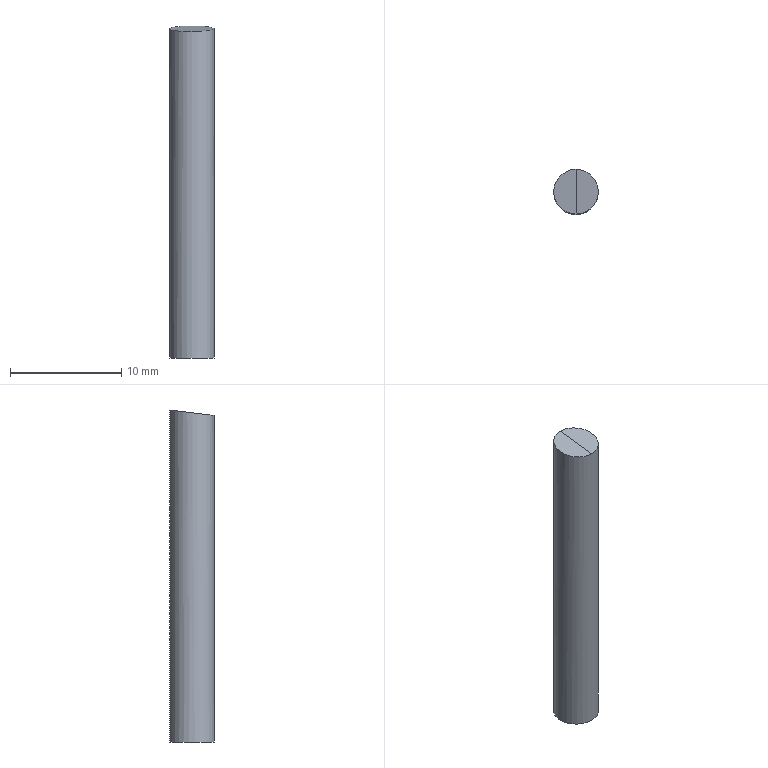Part | NX | features solid 2 | 1 solid | 4 faces | box 4 x 4 x 29.794 mm | volume 371.265 mm3 | plane 3 | cylinder 1 | commonest cylinder face diameters 4 x1
STEP:
#1=CARTESIAN_POINT('',(-0.00002254,-159.993,-1.));
#2=VERTEX_POINT('',#1);
#3=CARTESIAN_POINT('',(-0.00002254,-157.993,-1.));
#4=DIRECTION('',(0.,0.,1.));
#5=DIRECTION('',(0.,-1.,0.));
#6=AXIS2_PLACEMENT_3D('',#3,#4,#5);
#7=CIRCLE('',#6,2.);
#8=EDGE_CURVE('',#2,#2,#7,.T.);
#9=ORIENTED_EDGE('',*,*,#8,.F.);
#10=EDGE_LOOP('',(#9));
#11=FACE_BOUND('',#10,.T.);
#12=CARTESIAN_POINT('',(-0.00002254,-157.993,-1.));
#13=DIRECTION('',(0.,0.,-1.));
#14=DIRECTION('',(0.,1.,0.));
#15=AXIS2_PLACEMENT_3D('',#12,#13,#14);
#16=PLANE('',#15);
#17=ADVANCED_FACE('',(#11),#16,.T.);
#18=ORIENTED_EDGE('',*,*,#8,.T.);
#19=EDGE_LOOP('',(#18));
#20=FACE_BOUND('',#19,.T.);
#21=CARTESIAN_POINT('',(0.,-155.993,28.794));
#22=VERTEX_POINT('',#21);
#23=CARTESIAN_POINT('',(-0.00001127,-159.993,28.295));
#24=VERTEX_POINT('',#23);
#25=CARTESIAN_POINT('',(-0.00002254,-157.993,28.544));
#26=DIRECTION('',(0.,-0.1238,0.9923));
#27=DIRECTION('',(0.,-0.9923,-0.1238));
#28=AXIS2_PLACEMENT_3D('',#25,#26,#27);
#29=ELLIPSE('',#28,2.016,2.);
#30=EDGE_CURVE('',#22,#24,#29,.F.);
#31=ORIENTED_EDGE('',*,*,#30,.T.);
#32=CARTESIAN_POINT('',(-0.00002254,-157.993,28.544));
#33=DIRECTION('',(0.,-0.1238,0.9923));
#34=DIRECTION('',(0.,-0.9923,-0.1238));
#35=AXIS2_PLACEMENT_3D('',#32,#33,#34);
#36=ELLIPSE('',#35,2.016,2.);
#37=EDGE_CURVE('',#24,#22,#36,.F.);
#38=ORIENTED_EDGE('',*,*,#37,.T.);
#39=EDGE_LOOP('',(#31,#38));
#40=FACE_BOUND('',#39,.T.);
#41=CARTESIAN_POINT('',(-0.00002254,-157.993,29.));
#42=DIRECTION('',(0.,0.,-1.));
#43=DIRECTION('',(0.,1.,0.));
#44=AXIS2_PLACEMENT_3D('',#41,#42,#43);
#45=CYLINDRICAL_SURFACE('',#44,2.);
#46=ADVANCED_FACE('',(#20,#40),#45,.T.);
#47=ORIENTED_EDGE('',*,*,#30,.F.);
#48=CARTESIAN_POINT('',(0.,-155.993,28.794));
#49=CARTESIAN_POINT('',(0.,-157.326,28.628));
#50=CARTESIAN_POINT('',(0.,-158.659,28.461));
#51=CARTESIAN_POINT('',(0.,-159.993,28.295));
#52=B_SPLINE_CURVE_WITH_KNOTS('',3,(#48,#49,#50,#51),.UNSPECIFIED.,.F.,.F.,(4,4),(0.4639,0.611),.UNSPECIFIED.);
#53=EDGE_CURVE('',#24,#22,#52,.F.);
#54=ORIENTED_EDGE('',*,*,#53,.F.);
#55=EDGE_LOOP('',(#47,#54));
#56=FACE_BOUND('',#55,.T.);
#57=CARTESIAN_POINT('',(300.,-92.289,36.741));
#58=DIRECTION('',(0.,-0.1238,0.9923));
#59=DIRECTION('',(0.,0.9923,0.1238));
#60=AXIS2_PLACEMENT_3D('',#57,#58,#59);
#61=PLANE('',#60);
#62=ADVANCED_FACE('',(#56),#61,.T.);
#63=ORIENTED_EDGE('',*,*,#37,.F.);
#64=ORIENTED_EDGE('',*,*,#53,.T.);
#65=EDGE_LOOP('',(#63,#64));
#66=FACE_BOUND('',#65,.T.);
#67=CARTESIAN_POINT('',(-300.,-111.421,34.354));
#68=DIRECTION('',(0.,-0.1238,0.9923));
#69=DIRECTION('',(0.,0.9923,0.1238));
#70=AXIS2_PLACEMENT_3D('',#67,#68,#69);
#71=PLANE('',#70);
#72=ADVANCED_FACE('',(#66),#71,.T.);
#73=CLOSED_SHELL('',(#17,#46,#62,#72));
#74=MANIFOLD_SOLID_BREP('',#73);
#75=(LENGTH_UNIT()NAMED_UNIT(*)SI_UNIT(.MILLI.,.METRE.));
#76=UNCERTAINTY_MEASURE_WITH_UNIT(LENGTH_MEASURE(0.0508),#75,'','');
#77=(NAMED_UNIT(*)PLANE_ANGLE_UNIT()SI_UNIT($,.RADIAN.));
#78=(NAMED_UNIT(*)SI_UNIT($,.STERADIAN.)SOLID_ANGLE_UNIT());
#79=(GEOMETRIC_REPRESENTATION_CONTEXT(3)GLOBAL_UNCERTAINTY_ASSIGNED_CONTEXT((#76))GLOBAL_UNIT_ASSIGNED_CONTEXT((#75,#77,#78))REPRESENTATION_CONTEXT('',''));
#80=ADVANCED_BREP_SHAPE_REPRESENTATION('',(#74),#79);